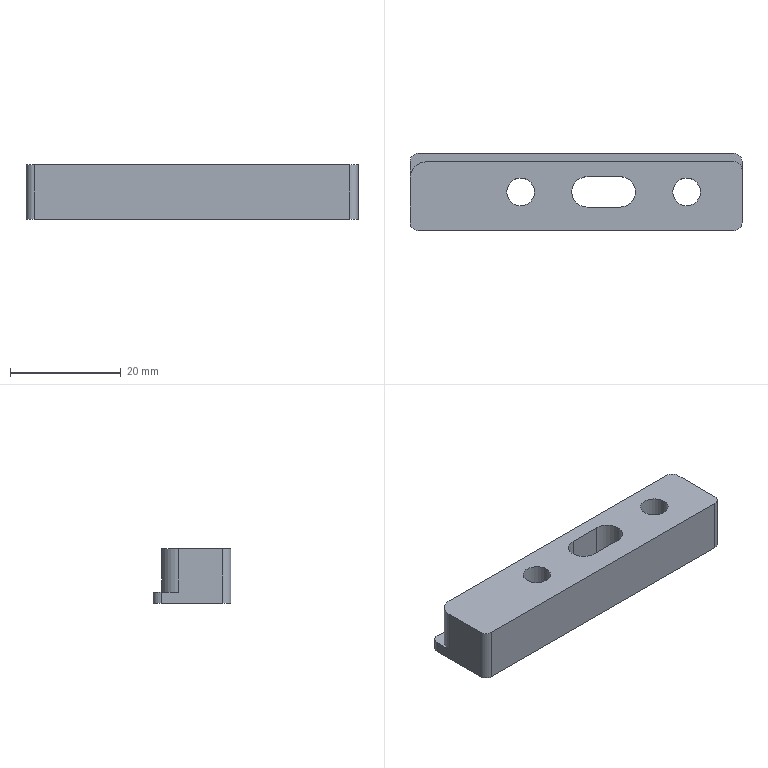Part | STEP file | 1 solid | 20 faces | box 60 x 14 x 9.8 mm | volume 6535 mm3 | plane 10 | cylinder 10 | commonest cylinder face diameters 3 x5 5 x2 5.5 x2 6 x1